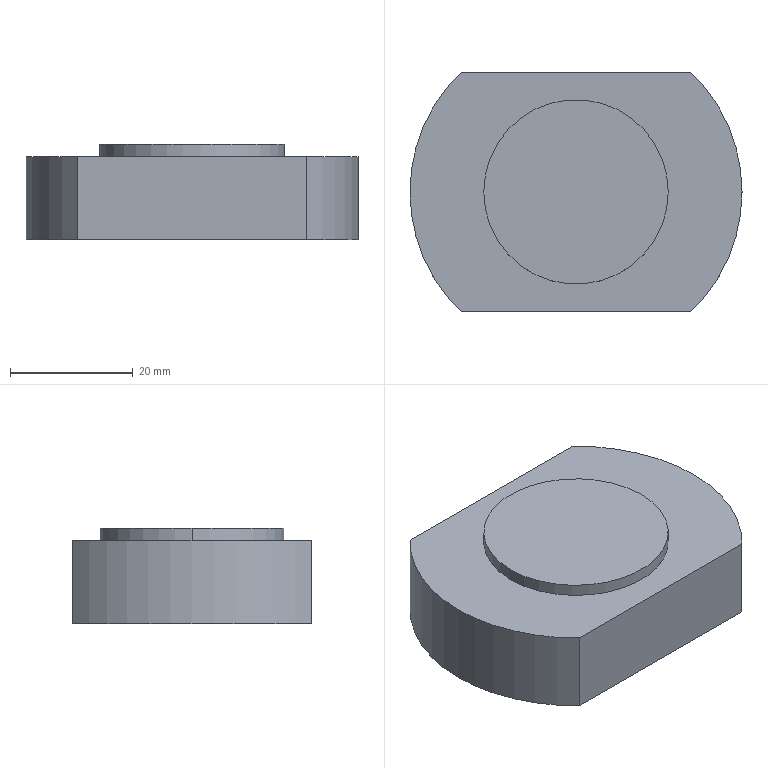Part | SolidWorks | features BaseBody 1 | 1 solid | 10 faces | box 54 x 39 x 15.5 mm | volume 27130 mm3 | cylinder 5 | plane 5 | commonest cylinder face diameters 54 x3 30 x2
STEP:
#1=CARTESIAN_POINT('',(27.,0.,-1.5));
#2=VERTEX_POINT('',#1);
#3=CARTESIAN_POINT('',(18.675,-19.5,-1.5));
#4=VERTEX_POINT('',#3);
#5=CARTESIAN_POINT('',(0.,0.,-1.5));
#6=DIRECTION('',(0.,0.,-1.));
#7=DIRECTION('',(1.,0.,0.));
#8=AXIS2_PLACEMENT_3D('',#5,#6,#7);
#9=CIRCLE('',#8,27.);
#10=EDGE_CURVE('',#2,#4,#9,.T.);
#11=ORIENTED_EDGE('',*,*,#10,.F.);
#12=CARTESIAN_POINT('',(27.,0.,12.));
#13=VERTEX_POINT('',#12);
#14=CARTESIAN_POINT('',(27.,0.,11.));
#15=DIRECTION('',(0.,0.,1.));
#16=VECTOR('',#15,1000.);
#17=LINE('',#14,#16);
#18=EDGE_CURVE('',#2,#13,#17,.T.);
#19=ORIENTED_EDGE('',*,*,#18,.T.);
#20=CARTESIAN_POINT('',(18.675,-19.5,12.));
#21=VERTEX_POINT('',#20);
#22=CARTESIAN_POINT('',(0.,0.,12.));
#23=DIRECTION('',(0.,0.,-1.));
#24=DIRECTION('',(1.,0.,0.));
#25=AXIS2_PLACEMENT_3D('',#22,#23,#24);
#26=CIRCLE('',#25,27.);
#27=EDGE_CURVE('',#13,#21,#26,.T.);
#28=ORIENTED_EDGE('',*,*,#27,.T.);
#29=CARTESIAN_POINT('',(18.675,-19.5,0.));
#30=DIRECTION('',(0.,0.,1.));
#31=VECTOR('',#30,1000.);
#32=LINE('',#29,#31);
#33=EDGE_CURVE('',#4,#21,#32,.T.);
#34=ORIENTED_EDGE('',*,*,#33,.F.);
#35=EDGE_LOOP('',(#11,#19,#28,#34));
#36=FACE_OUTER_BOUND('',#35,.T.);
#37=CARTESIAN_POINT('',(0.,0.,11.));
#38=DIRECTION('',(0.,0.,1.));
#39=DIRECTION('',(1.,0.,0.));
#40=AXIS2_PLACEMENT_3D('',#37,#38,#39);
#41=CYLINDRICAL_SURFACE('',#40,27.);
#42=ADVANCED_FACE('',(#36),#41,.T.);
#43=CARTESIAN_POINT('',(15.,0.,12.));
#44=VERTEX_POINT('',#43);
#45=CARTESIAN_POINT('',(-15.,0.,12.));
#46=VERTEX_POINT('',#45);
#47=CARTESIAN_POINT('',(0.,0.,12.));
#48=DIRECTION('',(0.,0.,1.));
#49=DIRECTION('',(1.,0.,0.));
#50=AXIS2_PLACEMENT_3D('',#47,#48,#49);
#51=CIRCLE('',#50,15.);
#52=EDGE_CURVE('',#44,#46,#51,.T.);
#53=ORIENTED_EDGE('',*,*,#52,.T.);
#54=CARTESIAN_POINT('',(-15.,0.,14.));
#55=VERTEX_POINT('',#54);
#56=CARTESIAN_POINT('',(-15.,0.,14.));
#57=DIRECTION('',(0.,0.,1.));
#58=VECTOR('',#57,1000.);
#59=LINE('',#56,#58);
#60=EDGE_CURVE('',#46,#55,#59,.T.);
#61=ORIENTED_EDGE('',*,*,#60,.T.);
#62=CARTESIAN_POINT('',(15.,0.,14.));
#63=VERTEX_POINT('',#62);
#64=CARTESIAN_POINT('',(0.,0.,14.));
#65=DIRECTION('',(0.,0.,-1.));
#66=DIRECTION('',(1.,0.,0.));
#67=AXIS2_PLACEMENT_3D('',#64,#65,#66);
#68=CIRCLE('',#67,15.);
#69=EDGE_CURVE('',#55,#63,#68,.T.);
#70=ORIENTED_EDGE('',*,*,#69,.T.);
#71=CARTESIAN_POINT('',(15.,0.,14.));
#72=DIRECTION('',(0.,0.,1.));
#73=VECTOR('',#72,1000.);
#74=LINE('',#71,#73);
#75=EDGE_CURVE('',#44,#63,#74,.T.);
#76=ORIENTED_EDGE('',*,*,#75,.F.);
#77=EDGE_LOOP('',(#53,#61,#70,#76));
#78=FACE_OUTER_BOUND('',#77,.T.);
#79=CARTESIAN_POINT('',(0.,0.,14.));
#80=DIRECTION('',(0.,0.,1.));
#81=DIRECTION('',(1.,0.,0.));
#82=AXIS2_PLACEMENT_3D('',#79,#80,#81);
#83=CYLINDRICAL_SURFACE('',#82,15.);
#84=ADVANCED_FACE('',(#78),#83,.T.);
#85=CARTESIAN_POINT('',(18.675,19.5,-1.5));
#86=VERTEX_POINT('',#85);
#87=CARTESIAN_POINT('',(0.,0.,-1.5));
#88=DIRECTION('',(0.,0.,-1.));
#89=DIRECTION('',(1.,0.,0.));
#90=AXIS2_PLACEMENT_3D('',#87,#88,#89);
#91=CIRCLE('',#90,27.);
#92=EDGE_CURVE('',#86,#2,#91,.T.);
#93=ORIENTED_EDGE('',*,*,#92,.T.);
#94=ORIENTED_EDGE('',*,*,#10,.T.);
#95=CARTESIAN_POINT('',(-18.675,-19.5,-1.5));
#96=VERTEX_POINT('',#95);
#97=CARTESIAN_POINT('',(0.,-19.5,-1.5));
#98=DIRECTION('',(-1.,0.,0.));
#99=VECTOR('',#98,1000.);
#100=LINE('',#97,#99);
#101=EDGE_CURVE('',#4,#96,#100,.T.);
#102=ORIENTED_EDGE('',*,*,#101,.T.);
#103=CARTESIAN_POINT('',(-18.675,19.5,-1.5));
#104=VERTEX_POINT('',#103);
#105=CARTESIAN_POINT('',(0.,0.,-1.5));
#106=DIRECTION('',(0.,0.,-1.));
#107=DIRECTION('',(1.,0.,0.));
#108=AXIS2_PLACEMENT_3D('',#105,#106,#107);
#109=CIRCLE('',#108,27.);
#110=EDGE_CURVE('',#96,#104,#109,.T.);
#111=ORIENTED_EDGE('',*,*,#110,.T.);
#112=CARTESIAN_POINT('',(0.,19.5,-1.5));
#113=DIRECTION('',(1.,0.,0.));
#114=VECTOR('',#113,1000.);
#115=LINE('',#112,#114);
#116=EDGE_CURVE('',#104,#86,#115,.T.);
#117=ORIENTED_EDGE('',*,*,#116,.T.);
#118=EDGE_LOOP('',(#93,#94,#102,#111,#117));
#119=FACE_OUTER_BOUND('',#118,.T.);
#120=CARTESIAN_POINT('',(0.,0.,-1.5));
#121=DIRECTION('',(0.,0.,-1.));
#122=DIRECTION('',(-1.,0.,0.));
#123=AXIS2_PLACEMENT_3D('',#120,#121,#122);
#124=PLANE('',#123);
#125=ADVANCED_FACE('',(#119),#124,.T.);
#126=ORIENTED_EDGE('',*,*,#33,.T.);
#127=CARTESIAN_POINT('',(-18.675,-19.5,12.));
#128=VERTEX_POINT('',#127);
#129=CARTESIAN_POINT('',(-25.,-19.5,12.));
#130=DIRECTION('',(-1.,0.,0.));
#131=VECTOR('',#130,1000.);
#132=LINE('',#129,#131);
#133=EDGE_CURVE('',#21,#128,#132,.T.);
#134=ORIENTED_EDGE('',*,*,#133,.T.);
#135=CARTESIAN_POINT('',(-18.675,-19.5,0.));
#136=DIRECTION('',(0.,0.,-1.));
#137=VECTOR('',#136,1000.);
#138=LINE('',#135,#137);
#139=EDGE_CURVE('',#128,#96,#138,.T.);
#140=ORIENTED_EDGE('',*,*,#139,.T.);
#141=ORIENTED_EDGE('',*,*,#101,.F.);
#142=EDGE_LOOP('',(#126,#134,#140,#141));
#143=FACE_OUTER_BOUND('',#142,.T.);
#144=CARTESIAN_POINT('',(-25.,-19.5,0.));
#145=DIRECTION('',(0.,-1.,0.));
#146=DIRECTION('',(0.,0.,-1.));
#147=AXIS2_PLACEMENT_3D('',#144,#145,#146);
#148=PLANE('',#147);
#149=ADVANCED_FACE('',(#143),#148,.T.);
#150=ORIENTED_EDGE('',*,*,#18,.F.);
#151=ORIENTED_EDGE('',*,*,#92,.F.);
#152=CARTESIAN_POINT('',(18.675,19.5,12.));
#153=VERTEX_POINT('',#152);
#154=CARTESIAN_POINT('',(18.675,19.5,11.));
#155=DIRECTION('',(0.,0.,1.));
#156=VECTOR('',#155,1000.);
#157=LINE('',#154,#156);
#158=EDGE_CURVE('',#86,#153,#157,.T.);
#159=ORIENTED_EDGE('',*,*,#158,.T.);
#160=CARTESIAN_POINT('',(0.,0.,12.));
#161=DIRECTION('',(0.,0.,-1.));
#162=DIRECTION('',(1.,0.,0.));
#163=AXIS2_PLACEMENT_3D('',#160,#161,#162);
#164=CIRCLE('',#163,27.);
#165=EDGE_CURVE('',#153,#13,#164,.T.);
#166=ORIENTED_EDGE('',*,*,#165,.T.);
#167=EDGE_LOOP('',(#150,#151,#159,#166));
#168=FACE_OUTER_BOUND('',#167,.T.);
#169=CARTESIAN_POINT('',(0.,0.,11.));
#170=DIRECTION('',(0.,0.,1.));
#171=DIRECTION('',(1.,0.,0.));
#172=AXIS2_PLACEMENT_3D('',#169,#170,#171);
#173=CYLINDRICAL_SURFACE('',#172,27.);
#174=ADVANCED_FACE('',(#168),#173,.T.);
#175=CARTESIAN_POINT('',(-18.675,19.5,12.));
#176=VERTEX_POINT('',#175);
#177=CARTESIAN_POINT('',(-18.675,19.5,0.));
#178=DIRECTION('',(0.,0.,1.));
#179=VECTOR('',#178,1000.);
#180=LINE('',#177,#179);
#181=EDGE_CURVE('',#104,#176,#180,.T.);
#182=ORIENTED_EDGE('',*,*,#181,.T.);
#183=CARTESIAN_POINT('',(25.,19.5,12.));
#184=DIRECTION('',(1.,0.,0.));
#185=VECTOR('',#184,1000.);
#186=LINE('',#183,#185);
#187=EDGE_CURVE('',#176,#153,#186,.T.);
#188=ORIENTED_EDGE('',*,*,#187,.T.);
#189=ORIENTED_EDGE('',*,*,#158,.F.);
#190=ORIENTED_EDGE('',*,*,#116,.F.);
#191=EDGE_LOOP('',(#182,#188,#189,#190));
#192=FACE_OUTER_BOUND('',#191,.T.);
#193=CARTESIAN_POINT('',(25.,19.5,0.));
#194=DIRECTION('',(0.,1.,0.));
#195=DIRECTION('',(0.,0.,1.));
#196=AXIS2_PLACEMENT_3D('',#193,#194,#195);
#197=PLANE('',#196);
#198=ADVANCED_FACE('',(#192),#197,.T.);
#199=ORIENTED_EDGE('',*,*,#139,.F.);
#200=CARTESIAN_POINT('',(0.,0.,12.));
#201=DIRECTION('',(0.,0.,-1.));
#202=DIRECTION('',(1.,0.,0.));
#203=AXIS2_PLACEMENT_3D('',#200,#201,#202);
#204=CIRCLE('',#203,27.);
#205=EDGE_CURVE('',#128,#176,#204,.T.);
#206=ORIENTED_EDGE('',*,*,#205,.T.);
#207=ORIENTED_EDGE('',*,*,#181,.F.);
#208=ORIENTED_EDGE('',*,*,#110,.F.);
#209=EDGE_LOOP('',(#199,#206,#207,#208));
#210=FACE_OUTER_BOUND('',#209,.T.);
#211=CARTESIAN_POINT('',(0.,0.,11.));
#212=DIRECTION('',(0.,0.,1.));
#213=DIRECTION('',(1.,0.,0.));
#214=AXIS2_PLACEMENT_3D('',#211,#212,#213);
#215=CYLINDRICAL_SURFACE('',#214,27.);
#216=ADVANCED_FACE('',(#210),#215,.T.);
#217=ORIENTED_EDGE('',*,*,#52,.F.);
#218=CARTESIAN_POINT('',(0.,0.,12.));
#219=DIRECTION('',(0.,0.,1.));
#220=DIRECTION('',(1.,0.,0.));
#221=AXIS2_PLACEMENT_3D('',#218,#219,#220);
#222=CIRCLE('',#221,15.);
#223=EDGE_CURVE('',#46,#44,#222,.T.);
#224=ORIENTED_EDGE('',*,*,#223,.F.);
#225=EDGE_LOOP('',(#217,#224));
#226=FACE_BOUND('',#225,.T.);
#227=ORIENTED_EDGE('',*,*,#165,.F.);
#228=ORIENTED_EDGE('',*,*,#187,.F.);
#229=ORIENTED_EDGE('',*,*,#205,.F.);
#230=ORIENTED_EDGE('',*,*,#133,.F.);
#231=ORIENTED_EDGE('',*,*,#27,.F.);
#232=EDGE_LOOP('',(#227,#228,#229,#230,#231));
#233=FACE_OUTER_BOUND('',#232,.T.);
#234=CARTESIAN_POINT('',(0.,0.,12.));
#235=DIRECTION('',(0.,0.,-1.));
#236=DIRECTION('',(-1.,0.,0.));
#237=AXIS2_PLACEMENT_3D('',#234,#235,#236);
#238=PLANE('',#237);
#239=ADVANCED_FACE('',(#226,#233),#238,.F.);
#240=ORIENTED_EDGE('',*,*,#60,.F.);
#241=ORIENTED_EDGE('',*,*,#223,.T.);
#242=ORIENTED_EDGE('',*,*,#75,.T.);
#243=CARTESIAN_POINT('',(0.,0.,14.));
#244=DIRECTION('',(0.,0.,-1.));
#245=DIRECTION('',(1.,0.,0.));
#246=AXIS2_PLACEMENT_3D('',#243,#244,#245);
#247=CIRCLE('',#246,15.);
#248=EDGE_CURVE('',#63,#55,#247,.T.);
#249=ORIENTED_EDGE('',*,*,#248,.T.);
#250=EDGE_LOOP('',(#240,#241,#242,#249));
#251=FACE_OUTER_BOUND('',#250,.T.);
#252=CARTESIAN_POINT('',(0.,0.,14.));
#253=DIRECTION('',(0.,0.,1.));
#254=DIRECTION('',(1.,0.,0.));
#255=AXIS2_PLACEMENT_3D('',#252,#253,#254);
#256=CYLINDRICAL_SURFACE('',#255,15.);
#257=ADVANCED_FACE('',(#251),#256,.T.);
#258=ORIENTED_EDGE('',*,*,#248,.F.);
#259=ORIENTED_EDGE('',*,*,#69,.F.);
#260=EDGE_LOOP('',(#258,#259));
#261=FACE_OUTER_BOUND('',#260,.T.);
#262=CARTESIAN_POINT('',(0.,0.,14.));
#263=DIRECTION('',(0.,0.,1.));
#264=DIRECTION('',(1.,0.,0.));
#265=AXIS2_PLACEMENT_3D('',#262,#263,#264);
#266=PLANE('',#265);
#267=ADVANCED_FACE('',(#261),#266,.T.);
#268=CLOSED_SHELL('',(#42,#84,#125,#149,#174,#198,#216,#239,#257,#267));
#269=MANIFOLD_SOLID_BREP('',#268);
#270=CARTESIAN_POINT('',(0.,0.,0.));
#271=DIRECTION('',(0.,0.,1.));
#272=DIRECTION('',(1.,0.,0.));
#273=AXIS2_PLACEMENT_3D('',#270,#271,#272);
#274=(LENGTH_UNIT()NAMED_UNIT(*)SI_UNIT(.MILLI.,.METRE.));
#275=UNCERTAINTY_MEASURE_WITH_UNIT(LENGTH_MEASURE(0.00001),#274,'','');
#276=(NAMED_UNIT(*)PLANE_ANGLE_UNIT()SI_UNIT($,.RADIAN.));
#277=(NAMED_UNIT(*)SI_UNIT($,.STERADIAN.)SOLID_ANGLE_UNIT());
#278=(GEOMETRIC_REPRESENTATION_CONTEXT(3)GLOBAL_UNCERTAINTY_ASSIGNED_CONTEXT((#275))GLOBAL_UNIT_ASSIGNED_CONTEXT((#274,#276,#277))REPRESENTATION_CONTEXT('',''));
#279=ADVANCED_BREP_SHAPE_REPRESENTATION('',(#269,#273),#278);